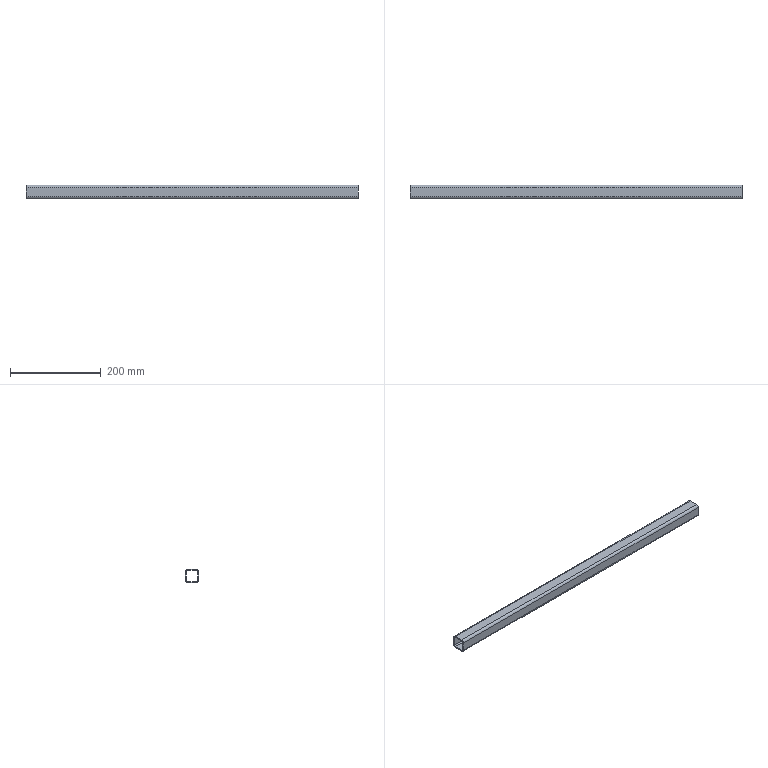Part | SolidWorks | features 3DProfileFeature 1, WeldMemberFeat 1, WeldmentFeature 1 | 1 solid | 18 faces | box 730 x 30 x 30 mm | volume 195313 mm3 | plane 10 | cylinder 8 | commonest cylinder face diameters 5.2 x4 10.4 x4
STEP:
#1=CARTESIAN_POINT('',(0.,9.8,-15.));
#2=VERTEX_POINT('',#1);
#3=CARTESIAN_POINT('',(0.,15.,-9.8));
#4=VERTEX_POINT('',#3);
#5=CARTESIAN_POINT('',(0.,9.8,-9.8));
#6=DIRECTION('',(1.,0.,0.));
#7=DIRECTION('',(0.,0.,-1.));
#8=AXIS2_PLACEMENT_3D('',#5,#6,#7);
#9=CIRCLE('',#8,5.2);
#10=EDGE_CURVE('',#2,#4,#9,.T.);
#11=ORIENTED_EDGE('',*,*,#10,.T.);
#12=CARTESIAN_POINT('',(730.,15.,-9.8));
#13=VERTEX_POINT('',#12);
#14=CARTESIAN_POINT('',(730.,15.,-9.8));
#15=DIRECTION('',(-1.,0.,0.));
#16=VECTOR('',#15,1000.);
#17=LINE('',#14,#16);
#18=EDGE_CURVE('',#13,#4,#17,.T.);
#19=ORIENTED_EDGE('',*,*,#18,.F.);
#20=CARTESIAN_POINT('',(730.,9.8,-15.));
#21=VERTEX_POINT('',#20);
#22=CARTESIAN_POINT('',(730.,9.8,-9.8));
#23=DIRECTION('',(1.,0.,0.));
#24=DIRECTION('',(0.,0.,-1.));
#25=AXIS2_PLACEMENT_3D('',#22,#23,#24);
#26=CIRCLE('',#25,5.2);
#27=EDGE_CURVE('',#21,#13,#26,.T.);
#28=ORIENTED_EDGE('',*,*,#27,.F.);
#29=CARTESIAN_POINT('',(730.,9.8,-15.));
#30=DIRECTION('',(-1.,0.,0.));
#31=VECTOR('',#30,1000.);
#32=LINE('',#29,#31);
#33=EDGE_CURVE('',#21,#2,#32,.T.);
#34=ORIENTED_EDGE('',*,*,#33,.T.);
#35=EDGE_LOOP('',(#11,#19,#28,#34));
#36=FACE_OUTER_BOUND('',#35,.T.);
#37=CARTESIAN_POINT('',(730.,9.8,-9.8));
#38=DIRECTION('',(-1.,0.,0.));
#39=DIRECTION('',(0.,0.,1.));
#40=AXIS2_PLACEMENT_3D('',#37,#38,#39);
#41=CYLINDRICAL_SURFACE('',#40,5.2);
#42=ADVANCED_FACE('',(#36),#41,.T.);
#43=CARTESIAN_POINT('',(0.,15.,9.8));
#44=VERTEX_POINT('',#43);
#45=CARTESIAN_POINT('',(0.,15.,-9.8));
#46=DIRECTION('',(0.,0.,1.));
#47=VECTOR('',#46,1000.);
#48=LINE('',#45,#47);
#49=EDGE_CURVE('',#4,#44,#48,.T.);
#50=ORIENTED_EDGE('',*,*,#49,.T.);
#51=CARTESIAN_POINT('',(730.,15.,9.8));
#52=VERTEX_POINT('',#51);
#53=CARTESIAN_POINT('',(730.,15.,9.8));
#54=DIRECTION('',(-1.,0.,0.));
#55=VECTOR('',#54,1000.);
#56=LINE('',#53,#55);
#57=EDGE_CURVE('',#52,#44,#56,.T.);
#58=ORIENTED_EDGE('',*,*,#57,.F.);
#59=CARTESIAN_POINT('',(730.,15.,-9.8));
#60=DIRECTION('',(0.,0.,1.));
#61=VECTOR('',#60,1000.);
#62=LINE('',#59,#61);
#63=EDGE_CURVE('',#13,#52,#62,.T.);
#64=ORIENTED_EDGE('',*,*,#63,.F.);
#65=ORIENTED_EDGE('',*,*,#18,.T.);
#66=EDGE_LOOP('',(#50,#58,#64,#65));
#67=FACE_OUTER_BOUND('',#66,.T.);
#68=CARTESIAN_POINT('',(730.,15.,-9.8));
#69=DIRECTION('',(0.,-1.,0.));
#70=DIRECTION('',(0.,0.,-1.));
#71=AXIS2_PLACEMENT_3D('',#68,#69,#70);
#72=PLANE('',#71);
#73=ADVANCED_FACE('',(#67),#72,.F.);
#74=CARTESIAN_POINT('',(0.,9.8,15.));
#75=VERTEX_POINT('',#74);
#76=CARTESIAN_POINT('',(0.,9.8,9.8));
#77=DIRECTION('',(1.,0.,0.));
#78=DIRECTION('',(0.,0.,-1.));
#79=AXIS2_PLACEMENT_3D('',#76,#77,#78);
#80=CIRCLE('',#79,5.2);
#81=EDGE_CURVE('',#44,#75,#80,.T.);
#82=ORIENTED_EDGE('',*,*,#81,.T.);
#83=CARTESIAN_POINT('',(730.,9.8,15.));
#84=VERTEX_POINT('',#83);
#85=CARTESIAN_POINT('',(730.,9.8,15.));
#86=DIRECTION('',(-1.,0.,0.));
#87=VECTOR('',#86,1000.);
#88=LINE('',#85,#87);
#89=EDGE_CURVE('',#84,#75,#88,.T.);
#90=ORIENTED_EDGE('',*,*,#89,.F.);
#91=CARTESIAN_POINT('',(730.,9.8,9.8));
#92=DIRECTION('',(1.,0.,0.));
#93=DIRECTION('',(0.,0.,-1.));
#94=AXIS2_PLACEMENT_3D('',#91,#92,#93);
#95=CIRCLE('',#94,5.2);
#96=EDGE_CURVE('',#52,#84,#95,.T.);
#97=ORIENTED_EDGE('',*,*,#96,.F.);
#98=ORIENTED_EDGE('',*,*,#57,.T.);
#99=EDGE_LOOP('',(#82,#90,#97,#98));
#100=FACE_OUTER_BOUND('',#99,.T.);
#101=CARTESIAN_POINT('',(730.,9.8,9.8));
#102=DIRECTION('',(-1.,0.,0.));
#103=DIRECTION('',(0.,0.,1.));
#104=AXIS2_PLACEMENT_3D('',#101,#102,#103);
#105=CYLINDRICAL_SURFACE('',#104,5.2);
#106=ADVANCED_FACE('',(#100),#105,.T.);
#107=CARTESIAN_POINT('',(0.,-9.8,15.));
#108=VERTEX_POINT('',#107);
#109=CARTESIAN_POINT('',(0.,-9.8,15.));
#110=DIRECTION('',(0.,-1.,0.));
#111=VECTOR('',#110,1000.);
#112=LINE('',#109,#111);
#113=EDGE_CURVE('',#75,#108,#112,.T.);
#114=ORIENTED_EDGE('',*,*,#113,.T.);
#115=CARTESIAN_POINT('',(730.,-9.8,15.));
#116=VERTEX_POINT('',#115);
#117=CARTESIAN_POINT('',(730.,-9.8,15.));
#118=DIRECTION('',(-1.,0.,0.));
#119=VECTOR('',#118,1000.);
#120=LINE('',#117,#119);
#121=EDGE_CURVE('',#116,#108,#120,.T.);
#122=ORIENTED_EDGE('',*,*,#121,.F.);
#123=CARTESIAN_POINT('',(730.,-9.8,15.));
#124=DIRECTION('',(0.,-1.,0.));
#125=VECTOR('',#124,1000.);
#126=LINE('',#123,#125);
#127=EDGE_CURVE('',#84,#116,#126,.T.);
#128=ORIENTED_EDGE('',*,*,#127,.F.);
#129=ORIENTED_EDGE('',*,*,#89,.T.);
#130=EDGE_LOOP('',(#114,#122,#128,#129));
#131=FACE_OUTER_BOUND('',#130,.T.);
#132=CARTESIAN_POINT('',(730.,-9.8,15.));
#133=DIRECTION('',(0.,0.,-1.));
#134=DIRECTION('',(-1.,0.,0.));
#135=AXIS2_PLACEMENT_3D('',#132,#133,#134);
#136=PLANE('',#135);
#137=ADVANCED_FACE('',(#131),#136,.F.);
#138=CARTESIAN_POINT('',(0.,-15.,9.8));
#139=VERTEX_POINT('',#138);
#140=CARTESIAN_POINT('',(0.,-9.8,9.8));
#141=DIRECTION('',(1.,0.,0.));
#142=DIRECTION('',(0.,0.,-1.));
#143=AXIS2_PLACEMENT_3D('',#140,#141,#142);
#144=CIRCLE('',#143,5.2);
#145=EDGE_CURVE('',#108,#139,#144,.T.);
#146=ORIENTED_EDGE('',*,*,#145,.T.);
#147=CARTESIAN_POINT('',(730.,-15.,9.8));
#148=VERTEX_POINT('',#147);
#149=CARTESIAN_POINT('',(730.,-15.,9.8));
#150=DIRECTION('',(-1.,0.,0.));
#151=VECTOR('',#150,1000.);
#152=LINE('',#149,#151);
#153=EDGE_CURVE('',#148,#139,#152,.T.);
#154=ORIENTED_EDGE('',*,*,#153,.F.);
#155=CARTESIAN_POINT('',(730.,-9.8,9.8));
#156=DIRECTION('',(1.,0.,0.));
#157=DIRECTION('',(0.,0.,-1.));
#158=AXIS2_PLACEMENT_3D('',#155,#156,#157);
#159=CIRCLE('',#158,5.2);
#160=EDGE_CURVE('',#116,#148,#159,.T.);
#161=ORIENTED_EDGE('',*,*,#160,.F.);
#162=ORIENTED_EDGE('',*,*,#121,.T.);
#163=EDGE_LOOP('',(#146,#154,#161,#162));
#164=FACE_OUTER_BOUND('',#163,.T.);
#165=CARTESIAN_POINT('',(730.,-9.8,9.8));
#166=DIRECTION('',(-1.,0.,0.));
#167=DIRECTION('',(0.,0.,1.));
#168=AXIS2_PLACEMENT_3D('',#165,#166,#167);
#169=CYLINDRICAL_SURFACE('',#168,5.2);
#170=ADVANCED_FACE('',(#164),#169,.T.);
#171=CARTESIAN_POINT('',(0.,-15.,-9.8));
#172=VERTEX_POINT('',#171);
#173=CARTESIAN_POINT('',(0.,-15.,9.8));
#174=DIRECTION('',(0.,0.,-1.));
#175=VECTOR('',#174,1000.);
#176=LINE('',#173,#175);
#177=EDGE_CURVE('',#139,#172,#176,.T.);
#178=ORIENTED_EDGE('',*,*,#177,.T.);
#179=CARTESIAN_POINT('',(730.,-15.,-9.8));
#180=VERTEX_POINT('',#179);
#181=CARTESIAN_POINT('',(730.,-15.,-9.8));
#182=DIRECTION('',(-1.,0.,0.));
#183=VECTOR('',#182,1000.);
#184=LINE('',#181,#183);
#185=EDGE_CURVE('',#180,#172,#184,.T.);
#186=ORIENTED_EDGE('',*,*,#185,.F.);
#187=CARTESIAN_POINT('',(730.,-15.,9.8));
#188=DIRECTION('',(0.,0.,-1.));
#189=VECTOR('',#188,1000.);
#190=LINE('',#187,#189);
#191=EDGE_CURVE('',#148,#180,#190,.T.);
#192=ORIENTED_EDGE('',*,*,#191,.F.);
#193=ORIENTED_EDGE('',*,*,#153,.T.);
#194=EDGE_LOOP('',(#178,#186,#192,#193));
#195=FACE_OUTER_BOUND('',#194,.T.);
#196=CARTESIAN_POINT('',(730.,-15.,9.8));
#197=DIRECTION('',(0.,1.,0.));
#198=DIRECTION('',(0.,0.,1.));
#199=AXIS2_PLACEMENT_3D('',#196,#197,#198);
#200=PLANE('',#199);
#201=ADVANCED_FACE('',(#195),#200,.F.);
#202=CARTESIAN_POINT('',(0.,-9.8,-15.));
#203=VERTEX_POINT('',#202);
#204=CARTESIAN_POINT('',(0.,-9.8,-9.8));
#205=DIRECTION('',(1.,0.,0.));
#206=DIRECTION('',(0.,0.,-1.));
#207=AXIS2_PLACEMENT_3D('',#204,#205,#206);
#208=CIRCLE('',#207,5.2);
#209=EDGE_CURVE('',#172,#203,#208,.T.);
#210=ORIENTED_EDGE('',*,*,#209,.T.);
#211=CARTESIAN_POINT('',(730.,-9.8,-15.));
#212=VERTEX_POINT('',#211);
#213=CARTESIAN_POINT('',(730.,-9.8,-15.));
#214=DIRECTION('',(-1.,0.,0.));
#215=VECTOR('',#214,1000.);
#216=LINE('',#213,#215);
#217=EDGE_CURVE('',#212,#203,#216,.T.);
#218=ORIENTED_EDGE('',*,*,#217,.F.);
#219=CARTESIAN_POINT('',(730.,-9.8,-9.8));
#220=DIRECTION('',(1.,0.,0.));
#221=DIRECTION('',(0.,0.,-1.));
#222=AXIS2_PLACEMENT_3D('',#219,#220,#221);
#223=CIRCLE('',#222,5.2);
#224=EDGE_CURVE('',#180,#212,#223,.T.);
#225=ORIENTED_EDGE('',*,*,#224,.F.);
#226=ORIENTED_EDGE('',*,*,#185,.T.);
#227=EDGE_LOOP('',(#210,#218,#225,#226));
#228=FACE_OUTER_BOUND('',#227,.T.);
#229=CARTESIAN_POINT('',(730.,-9.8,-9.8));
#230=DIRECTION('',(-1.,0.,0.));
#231=DIRECTION('',(0.,0.,1.));
#232=AXIS2_PLACEMENT_3D('',#229,#230,#231);
#233=CYLINDRICAL_SURFACE('',#232,5.2);
#234=ADVANCED_FACE('',(#228),#233,.T.);
#235=CARTESIAN_POINT('',(0.,12.4,9.8));
#236=VERTEX_POINT('',#235);
#237=CARTESIAN_POINT('',(0.,9.8,12.4));
#238=VERTEX_POINT('',#237);
#239=CARTESIAN_POINT('',(0.,9.8,9.8));
#240=DIRECTION('',(1.,0.,0.));
#241=DIRECTION('',(0.,0.,-1.));
#242=AXIS2_PLACEMENT_3D('',#239,#240,#241);
#243=CIRCLE('',#242,2.6);
#244=EDGE_CURVE('',#236,#238,#243,.T.);
#245=ORIENTED_EDGE('',*,*,#244,.F.);
#246=CARTESIAN_POINT('',(730.,12.4,9.8));
#247=VERTEX_POINT('',#246);
#248=CARTESIAN_POINT('',(730.,12.4,9.8));
#249=DIRECTION('',(-1.,0.,0.));
#250=VECTOR('',#249,1000.);
#251=LINE('',#248,#250);
#252=EDGE_CURVE('',#247,#236,#251,.T.);
#253=ORIENTED_EDGE('',*,*,#252,.F.);
#254=CARTESIAN_POINT('',(730.,9.8,12.4));
#255=VERTEX_POINT('',#254);
#256=CARTESIAN_POINT('',(730.,9.8,9.8));
#257=DIRECTION('',(1.,0.,0.));
#258=DIRECTION('',(0.,0.,-1.));
#259=AXIS2_PLACEMENT_3D('',#256,#257,#258);
#260=CIRCLE('',#259,2.6);
#261=EDGE_CURVE('',#247,#255,#260,.T.);
#262=ORIENTED_EDGE('',*,*,#261,.T.);
#263=CARTESIAN_POINT('',(730.,9.8,12.4));
#264=DIRECTION('',(-1.,0.,0.));
#265=VECTOR('',#264,1000.);
#266=LINE('',#263,#265);
#267=EDGE_CURVE('',#255,#238,#266,.T.);
#268=ORIENTED_EDGE('',*,*,#267,.T.);
#269=EDGE_LOOP('',(#245,#253,#262,#268));
#270=FACE_OUTER_BOUND('',#269,.T.);
#271=CARTESIAN_POINT('',(730.,9.8,9.8));
#272=DIRECTION('',(-1.,0.,0.));
#273=DIRECTION('',(0.,0.,1.));
#274=AXIS2_PLACEMENT_3D('',#271,#272,#273);
#275=CYLINDRICAL_SURFACE('',#274,2.6);
#276=ADVANCED_FACE('',(#270),#275,.F.);
#277=CARTESIAN_POINT('',(0.,12.4,-9.8));
#278=VERTEX_POINT('',#277);
#279=CARTESIAN_POINT('',(0.,12.4,-9.8));
#280=DIRECTION('',(0.,0.,1.));
#281=VECTOR('',#280,1000.);
#282=LINE('',#279,#281);
#283=EDGE_CURVE('',#278,#236,#282,.T.);
#284=ORIENTED_EDGE('',*,*,#283,.F.);
#285=CARTESIAN_POINT('',(730.,12.4,-9.8));
#286=VERTEX_POINT('',#285);
#287=CARTESIAN_POINT('',(730.,12.4,-9.8));
#288=DIRECTION('',(-1.,0.,0.));
#289=VECTOR('',#288,1000.);
#290=LINE('',#287,#289);
#291=EDGE_CURVE('',#286,#278,#290,.T.);
#292=ORIENTED_EDGE('',*,*,#291,.F.);
#293=CARTESIAN_POINT('',(730.,12.4,-9.8));
#294=DIRECTION('',(0.,0.,1.));
#295=VECTOR('',#294,1000.);
#296=LINE('',#293,#295);
#297=EDGE_CURVE('',#286,#247,#296,.T.);
#298=ORIENTED_EDGE('',*,*,#297,.T.);
#299=ORIENTED_EDGE('',*,*,#252,.T.);
#300=EDGE_LOOP('',(#284,#292,#298,#299));
#301=FACE_OUTER_BOUND('',#300,.T.);
#302=CARTESIAN_POINT('',(730.,12.4,-9.8));
#303=DIRECTION('',(0.,-1.,0.));
#304=DIRECTION('',(0.,0.,-1.));
#305=AXIS2_PLACEMENT_3D('',#302,#303,#304);
#306=PLANE('',#305);
#307=ADVANCED_FACE('',(#301),#306,.T.);
#308=CARTESIAN_POINT('',(0.,9.8,-12.4));
#309=VERTEX_POINT('',#308);
#310=CARTESIAN_POINT('',(0.,9.8,-9.8));
#311=DIRECTION('',(1.,0.,0.));
#312=DIRECTION('',(0.,0.,-1.));
#313=AXIS2_PLACEMENT_3D('',#310,#311,#312);
#314=CIRCLE('',#313,2.6);
#315=EDGE_CURVE('',#309,#278,#314,.T.);
#316=ORIENTED_EDGE('',*,*,#315,.F.);
#317=CARTESIAN_POINT('',(730.,9.8,-12.4));
#318=VERTEX_POINT('',#317);
#319=CARTESIAN_POINT('',(730.,9.8,-12.4));
#320=DIRECTION('',(-1.,0.,0.));
#321=VECTOR('',#320,1000.);
#322=LINE('',#319,#321);
#323=EDGE_CURVE('',#318,#309,#322,.T.);
#324=ORIENTED_EDGE('',*,*,#323,.F.);
#325=CARTESIAN_POINT('',(730.,9.8,-9.8));
#326=DIRECTION('',(1.,0.,0.));
#327=DIRECTION('',(0.,0.,-1.));
#328=AXIS2_PLACEMENT_3D('',#325,#326,#327);
#329=CIRCLE('',#328,2.6);
#330=EDGE_CURVE('',#318,#286,#329,.T.);
#331=ORIENTED_EDGE('',*,*,#330,.T.);
#332=ORIENTED_EDGE('',*,*,#291,.T.);
#333=EDGE_LOOP('',(#316,#324,#331,#332));
#334=FACE_OUTER_BOUND('',#333,.T.);
#335=CARTESIAN_POINT('',(730.,9.8,-9.8));
#336=DIRECTION('',(-1.,0.,0.));
#337=DIRECTION('',(0.,0.,1.));
#338=AXIS2_PLACEMENT_3D('',#335,#336,#337);
#339=CYLINDRICAL_SURFACE('',#338,2.6);
#340=ADVANCED_FACE('',(#334),#339,.F.);
#341=CARTESIAN_POINT('',(0.,-9.8,-12.4));
#342=VERTEX_POINT('',#341);
#343=CARTESIAN_POINT('',(0.,9.8,-12.4));
#344=DIRECTION('',(0.,1.,0.));
#345=VECTOR('',#344,1000.);
#346=LINE('',#343,#345);
#347=EDGE_CURVE('',#342,#309,#346,.T.);
#348=ORIENTED_EDGE('',*,*,#347,.F.);
#349=CARTESIAN_POINT('',(730.,-9.8,-12.4));
#350=VERTEX_POINT('',#349);
#351=CARTESIAN_POINT('',(730.,-9.8,-12.4));
#352=DIRECTION('',(-1.,0.,0.));
#353=VECTOR('',#352,1000.);
#354=LINE('',#351,#353);
#355=EDGE_CURVE('',#350,#342,#354,.T.);
#356=ORIENTED_EDGE('',*,*,#355,.F.);
#357=CARTESIAN_POINT('',(730.,9.8,-12.4));
#358=DIRECTION('',(0.,1.,0.));
#359=VECTOR('',#358,1000.);
#360=LINE('',#357,#359);
#361=EDGE_CURVE('',#350,#318,#360,.T.);
#362=ORIENTED_EDGE('',*,*,#361,.T.);
#363=ORIENTED_EDGE('',*,*,#323,.T.);
#364=EDGE_LOOP('',(#348,#356,#362,#363));
#365=FACE_OUTER_BOUND('',#364,.T.);
#366=CARTESIAN_POINT('',(730.,9.8,-12.4));
#367=DIRECTION('',(0.,0.,1.));
#368=DIRECTION('',(1.,0.,0.));
#369=AXIS2_PLACEMENT_3D('',#366,#367,#368);
#370=PLANE('',#369);
#371=ADVANCED_FACE('',(#365),#370,.T.);
#372=CARTESIAN_POINT('',(0.,-12.4,-9.8));
#373=VERTEX_POINT('',#372);
#374=CARTESIAN_POINT('',(0.,-9.8,-9.8));
#375=DIRECTION('',(1.,0.,0.));
#376=DIRECTION('',(0.,0.,-1.));
#377=AXIS2_PLACEMENT_3D('',#374,#375,#376);
#378=CIRCLE('',#377,2.6);
#379=EDGE_CURVE('',#373,#342,#378,.T.);
#380=ORIENTED_EDGE('',*,*,#379,.F.);
#381=CARTESIAN_POINT('',(730.,-12.4,-9.8));
#382=VERTEX_POINT('',#381);
#383=CARTESIAN_POINT('',(730.,-12.4,-9.8));
#384=DIRECTION('',(-1.,0.,0.));
#385=VECTOR('',#384,1000.);
#386=LINE('',#383,#385);
#387=EDGE_CURVE('',#382,#373,#386,.T.);
#388=ORIENTED_EDGE('',*,*,#387,.F.);
#389=CARTESIAN_POINT('',(730.,-9.8,-9.8));
#390=DIRECTION('',(1.,0.,0.));
#391=DIRECTION('',(0.,0.,-1.));
#392=AXIS2_PLACEMENT_3D('',#389,#390,#391);
#393=CIRCLE('',#392,2.6);
#394=EDGE_CURVE('',#382,#350,#393,.T.);
#395=ORIENTED_EDGE('',*,*,#394,.T.);
#396=ORIENTED_EDGE('',*,*,#355,.T.);
#397=EDGE_LOOP('',(#380,#388,#395,#396));
#398=FACE_OUTER_BOUND('',#397,.T.);
#399=CARTESIAN_POINT('',(730.,-9.8,-9.8));
#400=DIRECTION('',(-1.,0.,0.));
#401=DIRECTION('',(0.,0.,1.));
#402=AXIS2_PLACEMENT_3D('',#399,#400,#401);
#403=CYLINDRICAL_SURFACE('',#402,2.6);
#404=ADVANCED_FACE('',(#398),#403,.F.);
#405=CARTESIAN_POINT('',(0.,-12.4,9.8));
#406=VERTEX_POINT('',#405);
#407=CARTESIAN_POINT('',(0.,-12.4,9.8));
#408=DIRECTION('',(0.,0.,-1.));
#409=VECTOR('',#408,1000.);
#410=LINE('',#407,#409);
#411=EDGE_CURVE('',#406,#373,#410,.T.);
#412=ORIENTED_EDGE('',*,*,#411,.F.);
#413=CARTESIAN_POINT('',(730.,-12.4,9.8));
#414=VERTEX_POINT('',#413);
#415=CARTESIAN_POINT('',(730.,-12.4,9.8));
#416=DIRECTION('',(-1.,0.,0.));
#417=VECTOR('',#416,1000.);
#418=LINE('',#415,#417);
#419=EDGE_CURVE('',#414,#406,#418,.T.);
#420=ORIENTED_EDGE('',*,*,#419,.F.);
#421=CARTESIAN_POINT('',(730.,-12.4,9.8));
#422=DIRECTION('',(0.,0.,-1.));
#423=VECTOR('',#422,1000.);
#424=LINE('',#421,#423);
#425=EDGE_CURVE('',#414,#382,#424,.T.);
#426=ORIENTED_EDGE('',*,*,#425,.T.);
#427=ORIENTED_EDGE('',*,*,#387,.T.);
#428=EDGE_LOOP('',(#412,#420,#426,#427));
#429=FACE_OUTER_BOUND('',#428,.T.);
#430=CARTESIAN_POINT('',(730.,-12.4,9.8));
#431=DIRECTION('',(0.,1.,0.));
#432=DIRECTION('',(0.,0.,1.));
#433=AXIS2_PLACEMENT_3D('',#430,#431,#432);
#434=PLANE('',#433);
#435=ADVANCED_FACE('',(#429),#434,.T.);
#436=CARTESIAN_POINT('',(0.,-9.8,12.4));
#437=VERTEX_POINT('',#436);
#438=CARTESIAN_POINT('',(0.,-9.8,9.8));
#439=DIRECTION('',(1.,0.,0.));
#440=DIRECTION('',(0.,0.,-1.));
#441=AXIS2_PLACEMENT_3D('',#438,#439,#440);
#442=CIRCLE('',#441,2.6);
#443=EDGE_CURVE('',#437,#406,#442,.T.);
#444=ORIENTED_EDGE('',*,*,#443,.F.);
#445=CARTESIAN_POINT('',(730.,-9.8,12.4));
#446=VERTEX_POINT('',#445);
#447=CARTESIAN_POINT('',(730.,-9.8,12.4));
#448=DIRECTION('',(-1.,0.,0.));
#449=VECTOR('',#448,1000.);
#450=LINE('',#447,#449);
#451=EDGE_CURVE('',#446,#437,#450,.T.);
#452=ORIENTED_EDGE('',*,*,#451,.F.);
#453=CARTESIAN_POINT('',(730.,-9.8,9.8));
#454=DIRECTION('',(1.,0.,0.));
#455=DIRECTION('',(0.,0.,-1.));
#456=AXIS2_PLACEMENT_3D('',#453,#454,#455);
#457=CIRCLE('',#456,2.6);
#458=EDGE_CURVE('',#446,#414,#457,.T.);
#459=ORIENTED_EDGE('',*,*,#458,.T.);
#460=ORIENTED_EDGE('',*,*,#419,.T.);
#461=EDGE_LOOP('',(#444,#452,#459,#460));
#462=FACE_OUTER_BOUND('',#461,.T.);
#463=CARTESIAN_POINT('',(730.,-9.8,9.8));
#464=DIRECTION('',(-1.,0.,0.));
#465=DIRECTION('',(0.,0.,1.));
#466=AXIS2_PLACEMENT_3D('',#463,#464,#465);
#467=CYLINDRICAL_SURFACE('',#466,2.6);
#468=ADVANCED_FACE('',(#462),#467,.F.);
#469=CARTESIAN_POINT('',(0.,-9.8,12.4));
#470=DIRECTION('',(0.,-1.,0.));
#471=VECTOR('',#470,1000.);
#472=LINE('',#469,#471);
#473=EDGE_CURVE('',#238,#437,#472,.T.);
#474=ORIENTED_EDGE('',*,*,#473,.F.);
#475=ORIENTED_EDGE('',*,*,#267,.F.);
#476=CARTESIAN_POINT('',(730.,-9.8,12.4));
#477=DIRECTION('',(0.,-1.,0.));
#478=VECTOR('',#477,1000.);
#479=LINE('',#476,#478);
#480=EDGE_CURVE('',#255,#446,#479,.T.);
#481=ORIENTED_EDGE('',*,*,#480,.T.);
#482=ORIENTED_EDGE('',*,*,#451,.T.);
#483=EDGE_LOOP('',(#474,#475,#481,#482));
#484=FACE_OUTER_BOUND('',#483,.T.);
#485=CARTESIAN_POINT('',(730.,-9.8,12.4));
#486=DIRECTION('',(0.,0.,-1.));
#487=DIRECTION('',(-1.,0.,0.));
#488=AXIS2_PLACEMENT_3D('',#485,#486,#487);
#489=PLANE('',#488);
#490=ADVANCED_FACE('',(#484),#489,.T.);
#491=CARTESIAN_POINT('',(0.,9.8,-15.));
#492=DIRECTION('',(0.,1.,0.));
#493=VECTOR('',#492,1000.);
#494=LINE('',#491,#493);
#495=EDGE_CURVE('',#203,#2,#494,.T.);
#496=ORIENTED_EDGE('',*,*,#495,.T.);
#497=ORIENTED_EDGE('',*,*,#33,.F.);
#498=CARTESIAN_POINT('',(730.,9.8,-15.));
#499=DIRECTION('',(0.,1.,0.));
#500=VECTOR('',#499,1000.);
#501=LINE('',#498,#500);
#502=EDGE_CURVE('',#212,#21,#501,.T.);
#503=ORIENTED_EDGE('',*,*,#502,.F.);
#504=ORIENTED_EDGE('',*,*,#217,.T.);
#505=EDGE_LOOP('',(#496,#497,#503,#504));
#506=FACE_OUTER_BOUND('',#505,.T.);
#507=CARTESIAN_POINT('',(730.,9.8,-15.));
#508=DIRECTION('',(0.,0.,1.));
#509=DIRECTION('',(1.,0.,0.));
#510=AXIS2_PLACEMENT_3D('',#507,#508,#509);
#511=PLANE('',#510);
#512=ADVANCED_FACE('',(#506),#511,.F.);
#513=ORIENTED_EDGE('',*,*,#261,.F.);
#514=ORIENTED_EDGE('',*,*,#297,.F.);
#515=ORIENTED_EDGE('',*,*,#330,.F.);
#516=ORIENTED_EDGE('',*,*,#361,.F.);
#517=ORIENTED_EDGE('',*,*,#394,.F.);
#518=ORIENTED_EDGE('',*,*,#425,.F.);
#519=ORIENTED_EDGE('',*,*,#458,.F.);
#520=ORIENTED_EDGE('',*,*,#480,.F.);
#521=EDGE_LOOP('',(#513,#514,#515,#516,#517,#518,#519,#520));
#522=FACE_BOUND('',#521,.T.);
#523=ORIENTED_EDGE('',*,*,#27,.T.);
#524=ORIENTED_EDGE('',*,*,#63,.T.);
#525=ORIENTED_EDGE('',*,*,#96,.T.);
#526=ORIENTED_EDGE('',*,*,#127,.T.);
#527=ORIENTED_EDGE('',*,*,#160,.T.);
#528=ORIENTED_EDGE('',*,*,#191,.T.);
#529=ORIENTED_EDGE('',*,*,#224,.T.);
#530=ORIENTED_EDGE('',*,*,#502,.T.);
#531=EDGE_LOOP('',(#523,#524,#525,#526,#527,#528,#529,#530));
#532=FACE_OUTER_BOUND('',#531,.T.);
#533=CARTESIAN_POINT('',(730.,9.8,-9.8));
#534=DIRECTION('',(1.,0.,0.));
#535=DIRECTION('',(0.,0.,-1.));
#536=AXIS2_PLACEMENT_3D('',#533,#534,#535);
#537=PLANE('',#536);
#538=ADVANCED_FACE('',(#522,#532),#537,.T.);
#539=ORIENTED_EDGE('',*,*,#244,.T.);
#540=ORIENTED_EDGE('',*,*,#473,.T.);
#541=ORIENTED_EDGE('',*,*,#443,.T.);
#542=ORIENTED_EDGE('',*,*,#411,.T.);
#543=ORIENTED_EDGE('',*,*,#379,.T.);
#544=ORIENTED_EDGE('',*,*,#347,.T.);
#545=ORIENTED_EDGE('',*,*,#315,.T.);
#546=ORIENTED_EDGE('',*,*,#283,.T.);
#547=EDGE_LOOP('',(#539,#540,#541,#542,#543,#544,#545,#546));
#548=FACE_BOUND('',#547,.T.);
#549=ORIENTED_EDGE('',*,*,#10,.F.);
#550=ORIENTED_EDGE('',*,*,#495,.F.);
#551=ORIENTED_EDGE('',*,*,#209,.F.);
#552=ORIENTED_EDGE('',*,*,#177,.F.);
#553=ORIENTED_EDGE('',*,*,#145,.F.);
#554=ORIENTED_EDGE('',*,*,#113,.F.);
#555=ORIENTED_EDGE('',*,*,#81,.F.);
#556=ORIENTED_EDGE('',*,*,#49,.F.);
#557=EDGE_LOOP('',(#549,#550,#551,#552,#553,#554,#555,#556));
#558=FACE_OUTER_BOUND('',#557,.T.);
#559=CARTESIAN_POINT('',(0.,9.8,-9.8));
#560=DIRECTION('',(1.,0.,0.));
#561=DIRECTION('',(0.,0.,-1.));
#562=AXIS2_PLACEMENT_3D('',#559,#560,#561);
#563=PLANE('',#562);
#564=ADVANCED_FACE('',(#548,#558),#563,.F.);
#565=CLOSED_SHELL('',(#42,#73,#106,#137,#170,#201,#234,#276,#307,#340,#371,#404,#435,#468,#490,#512,#538,#564));
#566=MANIFOLD_SOLID_BREP('',#565);
#567=CARTESIAN_POINT('',(0.,0.,0.));
#568=DIRECTION('',(0.,0.,1.));
#569=DIRECTION('',(1.,0.,0.));
#570=AXIS2_PLACEMENT_3D('',#567,#568,#569);
#571=(LENGTH_UNIT()NAMED_UNIT(*)SI_UNIT(.MILLI.,.METRE.));
#572=UNCERTAINTY_MEASURE_WITH_UNIT(LENGTH_MEASURE(0.00001),#571,'','');
#573=(NAMED_UNIT(*)PLANE_ANGLE_UNIT()SI_UNIT($,.RADIAN.));
#574=(NAMED_UNIT(*)SI_UNIT($,.STERADIAN.)SOLID_ANGLE_UNIT());
#575=(GEOMETRIC_REPRESENTATION_CONTEXT(3)GLOBAL_UNCERTAINTY_ASSIGNED_CONTEXT((#572))GLOBAL_UNIT_ASSIGNED_CONTEXT((#571,#573,#574))REPRESENTATION_CONTEXT('',''));
#576=ADVANCED_BREP_SHAPE_REPRESENTATION('',(#566,#570),#575);